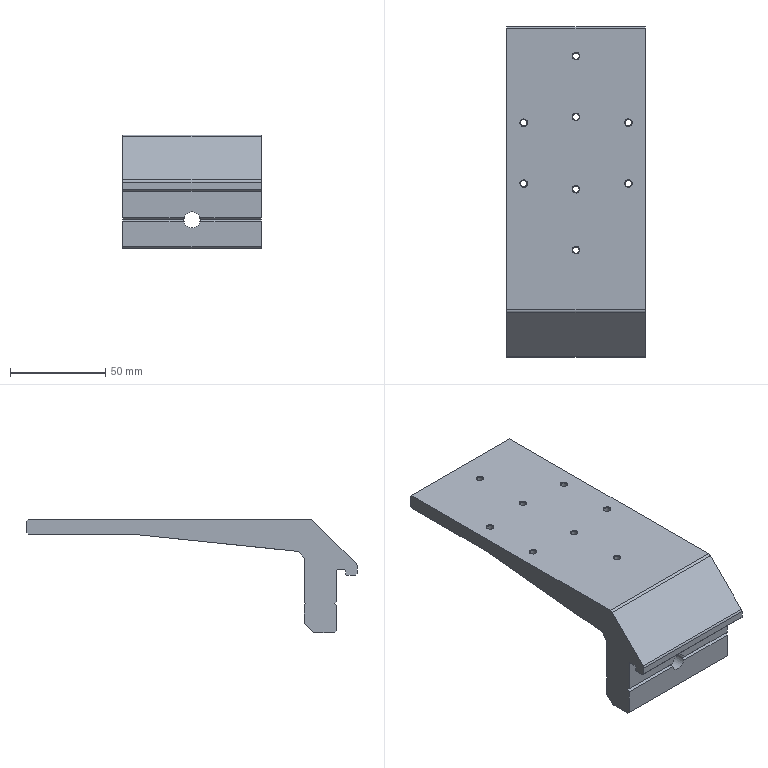Part | NX | features SIMPLE HOLE 8, SYMBOLIC_THREAD 8, DATUM_CSYS 3, EXTRUDE 2, SKETCH 2, HOLE PACKAGE 1 | 1 solid | 60 faces | box 73 x 173.8 x 59.75 mm | volume 188339 mm3 | plane 33 | cone 12 | cylinder 11 | spline 4 | commonest cylinder face diameters 3.3 x8 4 x2 8.5 x1